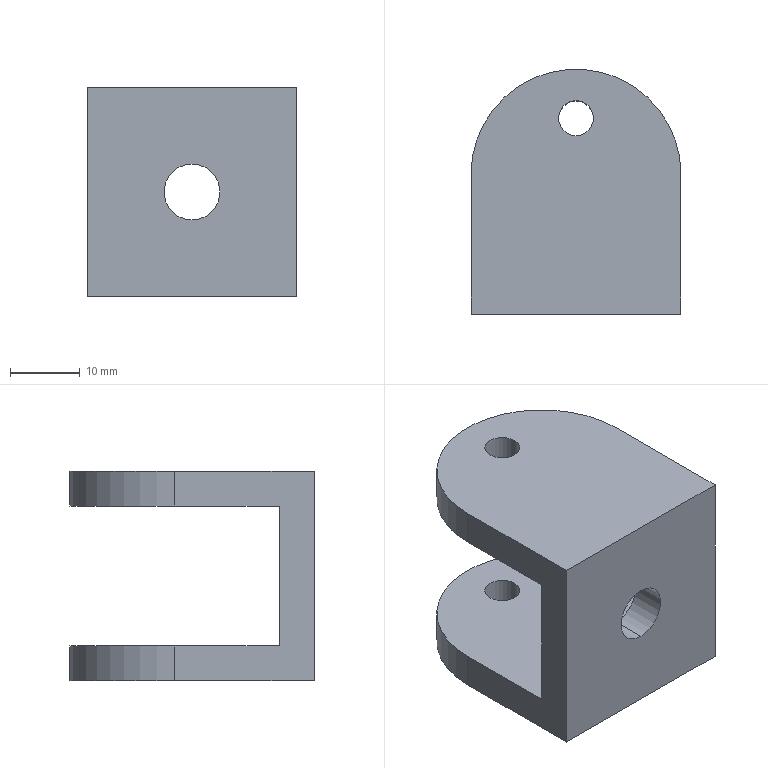Part | SolidWorks | features ICE 4, Extrusion 1 | 1 solid | 16 faces | box 30 x 35 x 30 mm | volume 12087 mm3 | cylinder 8 | plane 8 | commonest cylinder face diameters 5 x4 8 x2 30 x2
STEP:
#1=CARTESIAN_POINT('',(15.,5.,19.));
#2=VERTEX_POINT('',#1);
#3=CARTESIAN_POINT('',(15.,5.,11.));
#4=VERTEX_POINT('',#3);
#5=CARTESIAN_POINT('',(15.,5.,15.));
#6=DIRECTION('',(0.,-1.,0.));
#7=DIRECTION('',(1.,0.,0.));
#8=AXIS2_PLACEMENT_3D('',#5,#6,#7);
#9=CIRCLE('',#8,4.);
#10=EDGE_CURVE('',#2,#4,#9,.T.);
#11=ORIENTED_EDGE('',*,*,#10,.F.);
#12=CARTESIAN_POINT('',(15.,0.,19.));
#13=VERTEX_POINT('',#12);
#14=CARTESIAN_POINT('',(15.,40.,19.));
#15=DIRECTION('',(0.,-1.,0.));
#16=VECTOR('',#15,1000.);
#17=LINE('',#14,#16);
#18=EDGE_CURVE('',#2,#13,#17,.T.);
#19=ORIENTED_EDGE('',*,*,#18,.T.);
#20=CARTESIAN_POINT('',(15.,0.,11.));
#21=VERTEX_POINT('',#20);
#22=CARTESIAN_POINT('',(15.,0.,15.));
#23=DIRECTION('',(0.,-1.,0.));
#24=DIRECTION('',(0.,0.,-1.));
#25=AXIS2_PLACEMENT_3D('',#22,#23,#24);
#26=CIRCLE('',#25,4.);
#27=EDGE_CURVE('',#13,#21,#26,.T.);
#28=ORIENTED_EDGE('',*,*,#27,.T.);
#29=CARTESIAN_POINT('',(15.,40.,11.));
#30=DIRECTION('',(0.,-1.,0.));
#31=VECTOR('',#30,1000.);
#32=LINE('',#29,#31);
#33=EDGE_CURVE('',#4,#21,#32,.T.);
#34=ORIENTED_EDGE('',*,*,#33,.F.);
#35=EDGE_LOOP('',(#11,#19,#28,#34));
#36=FACE_OUTER_BOUND('',#35,.T.);
#37=CARTESIAN_POINT('',(15.,40.,15.));
#38=DIRECTION('',(0.,-1.,0.));
#39=DIRECTION('',(0.,0.,-1.));
#40=AXIS2_PLACEMENT_3D('',#37,#38,#39);
#41=CYLINDRICAL_SURFACE('',#40,4.);
#42=ADVANCED_FACE('',(#36),#41,.F.);
#43=CARTESIAN_POINT('',(17.5,28.,30.));
#44=VERTEX_POINT('',#43);
#45=CARTESIAN_POINT('',(12.5,28.,30.));
#46=VERTEX_POINT('',#45);
#47=CARTESIAN_POINT('',(15.,28.,30.));
#48=DIRECTION('',(0.,0.,-1.));
#49=DIRECTION('',(-1.,0.,0.));
#50=AXIS2_PLACEMENT_3D('',#47,#48,#49);
#51=CIRCLE('',#50,2.5);
#52=EDGE_CURVE('',#44,#46,#51,.T.);
#53=ORIENTED_EDGE('',*,*,#52,.F.);
#54=CARTESIAN_POINT('',(17.5,28.,25.));
#55=VERTEX_POINT('',#54);
#56=CARTESIAN_POINT('',(17.5,28.,40.));
#57=DIRECTION('',(0.,0.,-1.));
#58=VECTOR('',#57,1000.);
#59=LINE('',#56,#58);
#60=EDGE_CURVE('',#44,#55,#59,.T.);
#61=ORIENTED_EDGE('',*,*,#60,.T.);
#62=CARTESIAN_POINT('',(12.5,28.,25.));
#63=VERTEX_POINT('',#62);
#64=CARTESIAN_POINT('',(15.,28.,25.));
#65=DIRECTION('',(0.,0.,1.));
#66=DIRECTION('',(1.,0.,0.));
#67=AXIS2_PLACEMENT_3D('',#64,#65,#66);
#68=CIRCLE('',#67,2.5);
#69=EDGE_CURVE('',#63,#55,#68,.T.);
#70=ORIENTED_EDGE('',*,*,#69,.F.);
#71=CARTESIAN_POINT('',(12.5,28.,40.));
#72=DIRECTION('',(0.,0.,-1.));
#73=VECTOR('',#72,1000.);
#74=LINE('',#71,#73);
#75=EDGE_CURVE('',#46,#63,#74,.T.);
#76=ORIENTED_EDGE('',*,*,#75,.F.);
#77=EDGE_LOOP('',(#53,#61,#70,#76));
#78=FACE_OUTER_BOUND('',#77,.T.);
#79=CARTESIAN_POINT('',(15.,28.,40.));
#80=DIRECTION('',(0.,0.,-1.));
#81=DIRECTION('',(-1.,0.,0.));
#82=AXIS2_PLACEMENT_3D('',#79,#80,#81);
#83=CYLINDRICAL_SURFACE('',#82,2.5);
#84=ADVANCED_FACE('',(#78),#83,.F.);
#85=CARTESIAN_POINT('',(17.5,28.,5.));
#86=VERTEX_POINT('',#85);
#87=CARTESIAN_POINT('',(12.5,28.,5.));
#88=VERTEX_POINT('',#87);
#89=CARTESIAN_POINT('',(15.,28.,5.));
#90=DIRECTION('',(0.,0.,-1.));
#91=DIRECTION('',(0.,1.,0.));
#92=AXIS2_PLACEMENT_3D('',#89,#90,#91);
#93=CIRCLE('',#92,2.5);
#94=EDGE_CURVE('',#86,#88,#93,.T.);
#95=ORIENTED_EDGE('',*,*,#94,.F.);
#96=CARTESIAN_POINT('',(17.5,28.,0.));
#97=VERTEX_POINT('',#96);
#98=CARTESIAN_POINT('',(17.5,28.,40.));
#99=DIRECTION('',(0.,0.,-1.));
#100=VECTOR('',#99,1000.);
#101=LINE('',#98,#100);
#102=EDGE_CURVE('',#86,#97,#101,.T.);
#103=ORIENTED_EDGE('',*,*,#102,.T.);
#104=CARTESIAN_POINT('',(12.5,28.,0.));
#105=VERTEX_POINT('',#104);
#106=CARTESIAN_POINT('',(15.,28.,0.));
#107=DIRECTION('',(0.,0.,-1.));
#108=DIRECTION('',(-1.,0.,0.));
#109=AXIS2_PLACEMENT_3D('',#106,#107,#108);
#110=CIRCLE('',#109,2.5);
#111=EDGE_CURVE('',#97,#105,#110,.T.);
#112=ORIENTED_EDGE('',*,*,#111,.T.);
#113=CARTESIAN_POINT('',(12.5,28.,40.));
#114=DIRECTION('',(0.,0.,-1.));
#115=VECTOR('',#114,1000.);
#116=LINE('',#113,#115);
#117=EDGE_CURVE('',#88,#105,#116,.T.);
#118=ORIENTED_EDGE('',*,*,#117,.F.);
#119=EDGE_LOOP('',(#95,#103,#112,#118));
#120=FACE_OUTER_BOUND('',#119,.T.);
#121=CARTESIAN_POINT('',(15.,28.,40.));
#122=DIRECTION('',(0.,0.,-1.));
#123=DIRECTION('',(-1.,0.,0.));
#124=AXIS2_PLACEMENT_3D('',#121,#122,#123);
#125=CYLINDRICAL_SURFACE('',#124,2.5);
#126=ADVANCED_FACE('',(#120),#125,.F.);
#127=CARTESIAN_POINT('',(0.,20.,5.));
#128=VERTEX_POINT('',#127);
#129=CARTESIAN_POINT('',(0.,20.,0.));
#130=VERTEX_POINT('',#129);
#131=CARTESIAN_POINT('',(0.,20.,40.));
#132=DIRECTION('',(0.,0.,-1.));
#133=VECTOR('',#132,1000.);
#134=LINE('',#131,#133);
#135=EDGE_CURVE('',#128,#130,#134,.T.);
#136=ORIENTED_EDGE('',*,*,#135,.T.);
#137=CARTESIAN_POINT('',(0.,0.,0.));
#138=VERTEX_POINT('',#137);
#139=CARTESIAN_POINT('',(0.,0.,0.));
#140=DIRECTION('',(0.,-1.,0.));
#141=VECTOR('',#140,1000.);
#142=LINE('',#139,#141);
#143=EDGE_CURVE('',#130,#138,#142,.T.);
#144=ORIENTED_EDGE('',*,*,#143,.T.);
#145=CARTESIAN_POINT('',(0.,0.,30.));
#146=VERTEX_POINT('',#145);
#147=CARTESIAN_POINT('',(0.,0.,30.));
#148=DIRECTION('',(0.,0.,-1.));
#149=VECTOR('',#148,1000.);
#150=LINE('',#147,#149);
#151=EDGE_CURVE('',#146,#138,#150,.T.);
#152=ORIENTED_EDGE('',*,*,#151,.F.);
#153=CARTESIAN_POINT('',(0.,20.,30.));
#154=VERTEX_POINT('',#153);
#155=CARTESIAN_POINT('',(0.,0.,30.));
#156=DIRECTION('',(0.,-1.,0.));
#157=VECTOR('',#156,1000.);
#158=LINE('',#155,#157);
#159=EDGE_CURVE('',#154,#146,#158,.T.);
#160=ORIENTED_EDGE('',*,*,#159,.F.);
#161=CARTESIAN_POINT('',(0.,20.,25.));
#162=VERTEX_POINT('',#161);
#163=CARTESIAN_POINT('',(0.,20.,40.));
#164=DIRECTION('',(0.,0.,-1.));
#165=VECTOR('',#164,1000.);
#166=LINE('',#163,#165);
#167=EDGE_CURVE('',#154,#162,#166,.T.);
#168=ORIENTED_EDGE('',*,*,#167,.T.);
#169=CARTESIAN_POINT('',(0.,5.,25.));
#170=VERTEX_POINT('',#169);
#171=CARTESIAN_POINT('',(0.,0.,25.));
#172=DIRECTION('',(0.,-1.,0.));
#173=VECTOR('',#172,1000.);
#174=LINE('',#171,#173);
#175=EDGE_CURVE('',#162,#170,#174,.T.);
#176=ORIENTED_EDGE('',*,*,#175,.T.);
#177=CARTESIAN_POINT('',(0.,5.,5.));
#178=VERTEX_POINT('',#177);
#179=CARTESIAN_POINT('',(0.,5.,30.));
#180=DIRECTION('',(0.,0.,-1.));
#181=VECTOR('',#180,1000.);
#182=LINE('',#179,#181);
#183=EDGE_CURVE('',#170,#178,#182,.T.);
#184=ORIENTED_EDGE('',*,*,#183,.T.);
#185=CARTESIAN_POINT('',(0.,0.,5.));
#186=DIRECTION('',(0.,1.,0.));
#187=VECTOR('',#186,1000.);
#188=LINE('',#185,#187);
#189=EDGE_CURVE('',#178,#128,#188,.T.);
#190=ORIENTED_EDGE('',*,*,#189,.T.);
#191=EDGE_LOOP('',(#136,#144,#152,#160,#168,#176,#184,#190));
#192=FACE_OUTER_BOUND('',#191,.T.);
#193=CARTESIAN_POINT('',(0.,0.,30.));
#194=DIRECTION('',(1.,0.,0.));
#195=DIRECTION('',(0.,1.,0.));
#196=AXIS2_PLACEMENT_3D('',#193,#194,#195);
#197=PLANE('',#196);
#198=ADVANCED_FACE('',(#192),#197,.F.);
#199=CARTESIAN_POINT('',(15.,0.,15.));
#200=DIRECTION('',(0.,-1.,0.));
#201=DIRECTION('',(0.,0.,-1.));
#202=AXIS2_PLACEMENT_3D('',#199,#200,#201);
#203=CIRCLE('',#202,4.);
#204=EDGE_CURVE('',#21,#13,#203,.T.);
#205=ORIENTED_EDGE('',*,*,#204,.F.);
#206=ORIENTED_EDGE('',*,*,#27,.F.);
#207=EDGE_LOOP('',(#205,#206));
#208=FACE_BOUND('',#207,.T.);
#209=CARTESIAN_POINT('',(30.,0.,0.));
#210=VERTEX_POINT('',#209);
#211=CARTESIAN_POINT('',(0.,0.,0.));
#212=DIRECTION('',(1.,0.,0.));
#213=VECTOR('',#212,1000.);
#214=LINE('',#211,#213);
#215=EDGE_CURVE('',#138,#210,#214,.T.);
#216=ORIENTED_EDGE('',*,*,#215,.T.);
#217=CARTESIAN_POINT('',(30.,0.,30.));
#218=VERTEX_POINT('',#217);
#219=CARTESIAN_POINT('',(30.,0.,30.));
#220=DIRECTION('',(0.,0.,-1.));
#221=VECTOR('',#220,1000.);
#222=LINE('',#219,#221);
#223=EDGE_CURVE('',#218,#210,#222,.T.);
#224=ORIENTED_EDGE('',*,*,#223,.F.);
#225=CARTESIAN_POINT('',(0.,0.,30.));
#226=DIRECTION('',(1.,0.,0.));
#227=VECTOR('',#226,1000.);
#228=LINE('',#225,#227);
#229=EDGE_CURVE('',#146,#218,#228,.T.);
#230=ORIENTED_EDGE('',*,*,#229,.F.);
#231=ORIENTED_EDGE('',*,*,#151,.T.);
#232=EDGE_LOOP('',(#216,#224,#230,#231));
#233=FACE_OUTER_BOUND('',#232,.T.);
#234=CARTESIAN_POINT('',(0.,0.,30.));
#235=DIRECTION('',(0.,1.,0.));
#236=DIRECTION('',(0.,0.,1.));
#237=AXIS2_PLACEMENT_3D('',#234,#235,#236);
#238=PLANE('',#237);
#239=ADVANCED_FACE('',(#208,#233),#238,.F.);
#240=CARTESIAN_POINT('',(30.,20.,0.));
#241=VERTEX_POINT('',#240);
#242=CARTESIAN_POINT('',(30.,0.,0.));
#243=DIRECTION('',(0.,1.,0.));
#244=VECTOR('',#243,1000.);
#245=LINE('',#242,#244);
#246=EDGE_CURVE('',#210,#241,#245,.T.);
#247=ORIENTED_EDGE('',*,*,#246,.T.);
#248=CARTESIAN_POINT('',(30.,20.,5.));
#249=VERTEX_POINT('',#248);
#250=CARTESIAN_POINT('',(30.,20.,40.));
#251=DIRECTION('',(0.,0.,-1.));
#252=VECTOR('',#251,1000.);
#253=LINE('',#250,#252);
#254=EDGE_CURVE('',#249,#241,#253,.T.);
#255=ORIENTED_EDGE('',*,*,#254,.F.);
#256=CARTESIAN_POINT('',(30.,5.,5.));
#257=VERTEX_POINT('',#256);
#258=CARTESIAN_POINT('',(30.,40.,5.));
#259=DIRECTION('',(0.,1.,0.));
#260=VECTOR('',#259,1000.);
#261=LINE('',#258,#260);
#262=EDGE_CURVE('',#257,#249,#261,.T.);
#263=ORIENTED_EDGE('',*,*,#262,.F.);
#264=CARTESIAN_POINT('',(30.,5.,25.));
#265=VERTEX_POINT('',#264);
#266=CARTESIAN_POINT('',(30.,5.,25.));
#267=DIRECTION('',(0.,0.,-1.));
#268=VECTOR('',#267,1000.);
#269=LINE('',#266,#268);
#270=EDGE_CURVE('',#265,#257,#269,.T.);
#271=ORIENTED_EDGE('',*,*,#270,.F.);
#272=CARTESIAN_POINT('',(30.,20.,25.));
#273=VERTEX_POINT('',#272);
#274=CARTESIAN_POINT('',(30.,40.,25.));
#275=DIRECTION('',(0.,-1.,0.));
#276=VECTOR('',#275,1000.);
#277=LINE('',#274,#276);
#278=EDGE_CURVE('',#273,#265,#277,.T.);
#279=ORIENTED_EDGE('',*,*,#278,.F.);
#280=CARTESIAN_POINT('',(30.,20.,30.));
#281=VERTEX_POINT('',#280);
#282=CARTESIAN_POINT('',(30.,20.,40.));
#283=DIRECTION('',(0.,0.,-1.));
#284=VECTOR('',#283,1000.);
#285=LINE('',#282,#284);
#286=EDGE_CURVE('',#281,#273,#285,.T.);
#287=ORIENTED_EDGE('',*,*,#286,.F.);
#288=CARTESIAN_POINT('',(30.,0.,30.));
#289=DIRECTION('',(0.,1.,0.));
#290=VECTOR('',#289,1000.);
#291=LINE('',#288,#290);
#292=EDGE_CURVE('',#218,#281,#291,.T.);
#293=ORIENTED_EDGE('',*,*,#292,.F.);
#294=ORIENTED_EDGE('',*,*,#223,.T.);
#295=EDGE_LOOP('',(#247,#255,#263,#271,#279,#287,#293,#294));
#296=FACE_OUTER_BOUND('',#295,.T.);
#297=CARTESIAN_POINT('',(30.,0.,30.));
#298=DIRECTION('',(-1.,0.,0.));
#299=DIRECTION('',(0.,-1.,0.));
#300=AXIS2_PLACEMENT_3D('',#297,#298,#299);
#301=PLANE('',#300);
#302=ADVANCED_FACE('',(#296),#301,.F.);
#303=CARTESIAN_POINT('',(15.,28.,30.));
#304=DIRECTION('',(0.,0.,-1.));
#305=DIRECTION('',(-1.,0.,0.));
#306=AXIS2_PLACEMENT_3D('',#303,#304,#305);
#307=CIRCLE('',#306,2.5);
#308=EDGE_CURVE('',#46,#44,#307,.T.);
#309=ORIENTED_EDGE('',*,*,#308,.T.);
#310=ORIENTED_EDGE('',*,*,#52,.T.);
#311=EDGE_LOOP('',(#309,#310));
#312=FACE_BOUND('',#311,.T.);
#313=ORIENTED_EDGE('',*,*,#292,.T.);
#314=CARTESIAN_POINT('',(15.,20.,30.));
#315=DIRECTION('',(0.,0.,1.));
#316=DIRECTION('',(-1.,0.,0.));
#317=AXIS2_PLACEMENT_3D('',#314,#315,#316);
#318=CIRCLE('',#317,15.);
#319=EDGE_CURVE('',#281,#154,#318,.T.);
#320=ORIENTED_EDGE('',*,*,#319,.T.);
#321=ORIENTED_EDGE('',*,*,#159,.T.);
#322=ORIENTED_EDGE('',*,*,#229,.T.);
#323=EDGE_LOOP('',(#313,#320,#321,#322));
#324=FACE_OUTER_BOUND('',#323,.T.);
#325=CARTESIAN_POINT('',(0.,40.,30.));
#326=DIRECTION('',(0.,0.,-1.));
#327=DIRECTION('',(-1.,0.,0.));
#328=AXIS2_PLACEMENT_3D('',#325,#326,#327);
#329=PLANE('',#328);
#330=ADVANCED_FACE('',(#312,#324),#329,.F.);
#331=CARTESIAN_POINT('',(15.,28.,0.));
#332=DIRECTION('',(0.,0.,-1.));
#333=DIRECTION('',(-1.,0.,0.));
#334=AXIS2_PLACEMENT_3D('',#331,#332,#333);
#335=CIRCLE('',#334,2.5);
#336=EDGE_CURVE('',#105,#97,#335,.T.);
#337=ORIENTED_EDGE('',*,*,#336,.F.);
#338=ORIENTED_EDGE('',*,*,#111,.F.);
#339=EDGE_LOOP('',(#337,#338));
#340=FACE_BOUND('',#339,.T.);
#341=CARTESIAN_POINT('',(15.,20.,0.));
#342=DIRECTION('',(0.,0.,1.));
#343=DIRECTION('',(-1.,0.,0.));
#344=AXIS2_PLACEMENT_3D('',#341,#342,#343);
#345=CIRCLE('',#344,15.);
#346=EDGE_CURVE('',#241,#130,#345,.T.);
#347=ORIENTED_EDGE('',*,*,#346,.F.);
#348=ORIENTED_EDGE('',*,*,#246,.F.);
#349=ORIENTED_EDGE('',*,*,#215,.F.);
#350=ORIENTED_EDGE('',*,*,#143,.F.);
#351=EDGE_LOOP('',(#347,#348,#349,#350));
#352=FACE_OUTER_BOUND('',#351,.T.);
#353=CARTESIAN_POINT('',(0.,40.,0.));
#354=DIRECTION('',(0.,0.,-1.));
#355=DIRECTION('',(-1.,0.,0.));
#356=AXIS2_PLACEMENT_3D('',#353,#354,#355);
#357=PLANE('',#356);
#358=ADVANCED_FACE('',(#340,#352),#357,.T.);
#359=CARTESIAN_POINT('',(15.,5.,15.));
#360=DIRECTION('',(0.,-1.,0.));
#361=DIRECTION('',(1.,0.,0.));
#362=AXIS2_PLACEMENT_3D('',#359,#360,#361);
#363=CIRCLE('',#362,4.);
#364=EDGE_CURVE('',#4,#2,#363,.T.);
#365=ORIENTED_EDGE('',*,*,#364,.T.);
#366=ORIENTED_EDGE('',*,*,#10,.T.);
#367=EDGE_LOOP('',(#365,#366));
#368=FACE_BOUND('',#367,.T.);
#369=CARTESIAN_POINT('',(-10.,5.,25.));
#370=DIRECTION('',(1.,0.,0.));
#371=VECTOR('',#370,1000.);
#372=LINE('',#369,#371);
#373=EDGE_CURVE('',#170,#265,#372,.T.);
#374=ORIENTED_EDGE('',*,*,#373,.T.);
#375=ORIENTED_EDGE('',*,*,#270,.T.);
#376=CARTESIAN_POINT('',(-10.,5.,5.));
#377=DIRECTION('',(1.,0.,0.));
#378=VECTOR('',#377,1000.);
#379=LINE('',#376,#378);
#380=EDGE_CURVE('',#178,#257,#379,.T.);
#381=ORIENTED_EDGE('',*,*,#380,.F.);
#382=ORIENTED_EDGE('',*,*,#183,.F.);
#383=EDGE_LOOP('',(#374,#375,#381,#382));
#384=FACE_OUTER_BOUND('',#383,.T.);
#385=CARTESIAN_POINT('',(-10.,5.,25.));
#386=DIRECTION('',(0.,-1.,0.));
#387=DIRECTION('',(1.,0.,0.));
#388=AXIS2_PLACEMENT_3D('',#385,#386,#387);
#389=PLANE('',#388);
#390=ADVANCED_FACE('',(#368,#384),#389,.F.);
#391=ORIENTED_EDGE('',*,*,#69,.T.);
#392=CARTESIAN_POINT('',(15.,28.,25.));
#393=DIRECTION('',(0.,0.,1.));
#394=DIRECTION('',(1.,0.,0.));
#395=AXIS2_PLACEMENT_3D('',#392,#393,#394);
#396=CIRCLE('',#395,2.5);
#397=EDGE_CURVE('',#55,#63,#396,.T.);
#398=ORIENTED_EDGE('',*,*,#397,.T.);
#399=EDGE_LOOP('',(#391,#398));
#400=FACE_BOUND('',#399,.T.);
#401=ORIENTED_EDGE('',*,*,#175,.F.);
#402=CARTESIAN_POINT('',(15.,20.,25.));
#403=DIRECTION('',(0.,0.,-1.));
#404=DIRECTION('',(1.,0.,0.));
#405=AXIS2_PLACEMENT_3D('',#402,#403,#404);
#406=CIRCLE('',#405,15.);
#407=EDGE_CURVE('',#162,#273,#406,.T.);
#408=ORIENTED_EDGE('',*,*,#407,.T.);
#409=ORIENTED_EDGE('',*,*,#278,.T.);
#410=ORIENTED_EDGE('',*,*,#373,.F.);
#411=EDGE_LOOP('',(#401,#408,#409,#410));
#412=FACE_OUTER_BOUND('',#411,.T.);
#413=CARTESIAN_POINT('',(-10.,40.,25.));
#414=DIRECTION('',(0.,0.,1.));
#415=DIRECTION('',(1.,0.,0.));
#416=AXIS2_PLACEMENT_3D('',#413,#414,#415);
#417=PLANE('',#416);
#418=ADVANCED_FACE('',(#400,#412),#417,.F.);
#419=CARTESIAN_POINT('',(15.,28.,5.));
#420=DIRECTION('',(0.,0.,-1.));
#421=DIRECTION('',(0.,1.,0.));
#422=AXIS2_PLACEMENT_3D('',#419,#420,#421);
#423=CIRCLE('',#422,2.5);
#424=EDGE_CURVE('',#88,#86,#423,.T.);
#425=ORIENTED_EDGE('',*,*,#424,.T.);
#426=ORIENTED_EDGE('',*,*,#94,.T.);
#427=EDGE_LOOP('',(#425,#426));
#428=FACE_BOUND('',#427,.T.);
#429=ORIENTED_EDGE('',*,*,#262,.T.);
#430=CARTESIAN_POINT('',(15.,20.,5.));
#431=DIRECTION('',(0.,0.,1.));
#432=DIRECTION('',(0.,1.,0.));
#433=AXIS2_PLACEMENT_3D('',#430,#431,#432);
#434=CIRCLE('',#433,15.);
#435=EDGE_CURVE('',#249,#128,#434,.T.);
#436=ORIENTED_EDGE('',*,*,#435,.T.);
#437=ORIENTED_EDGE('',*,*,#189,.F.);
#438=ORIENTED_EDGE('',*,*,#380,.T.);
#439=EDGE_LOOP('',(#429,#436,#437,#438));
#440=FACE_OUTER_BOUND('',#439,.T.);
#441=CARTESIAN_POINT('',(-10.,40.,5.));
#442=DIRECTION('',(0.,0.,-1.));
#443=DIRECTION('',(0.,1.,0.));
#444=AXIS2_PLACEMENT_3D('',#441,#442,#443);
#445=PLANE('',#444);
#446=ADVANCED_FACE('',(#428,#440),#445,.F.);
#447=ORIENTED_EDGE('',*,*,#254,.T.);
#448=ORIENTED_EDGE('',*,*,#346,.T.);
#449=ORIENTED_EDGE('',*,*,#135,.F.);
#450=ORIENTED_EDGE('',*,*,#435,.F.);
#451=EDGE_LOOP('',(#447,#448,#449,#450));
#452=FACE_OUTER_BOUND('',#451,.T.);
#453=CARTESIAN_POINT('',(15.,20.,40.));
#454=DIRECTION('',(0.,0.,-1.));
#455=DIRECTION('',(-1.,0.,0.));
#456=AXIS2_PLACEMENT_3D('',#453,#454,#455);
#457=CYLINDRICAL_SURFACE('',#456,15.);
#458=ADVANCED_FACE('',(#452),#457,.T.);
#459=ORIENTED_EDGE('',*,*,#286,.T.);
#460=ORIENTED_EDGE('',*,*,#407,.F.);
#461=ORIENTED_EDGE('',*,*,#167,.F.);
#462=ORIENTED_EDGE('',*,*,#319,.F.);
#463=EDGE_LOOP('',(#459,#460,#461,#462));
#464=FACE_OUTER_BOUND('',#463,.T.);
#465=CARTESIAN_POINT('',(15.,20.,40.));
#466=DIRECTION('',(0.,0.,-1.));
#467=DIRECTION('',(-1.,0.,0.));
#468=AXIS2_PLACEMENT_3D('',#465,#466,#467);
#469=CYLINDRICAL_SURFACE('',#468,15.);
#470=ADVANCED_FACE('',(#464),#469,.T.);
#471=ORIENTED_EDGE('',*,*,#102,.F.);
#472=ORIENTED_EDGE('',*,*,#424,.F.);
#473=ORIENTED_EDGE('',*,*,#117,.T.);
#474=ORIENTED_EDGE('',*,*,#336,.T.);
#475=EDGE_LOOP('',(#471,#472,#473,#474));
#476=FACE_OUTER_BOUND('',#475,.T.);
#477=CARTESIAN_POINT('',(15.,28.,40.));
#478=DIRECTION('',(0.,0.,-1.));
#479=DIRECTION('',(-1.,0.,0.));
#480=AXIS2_PLACEMENT_3D('',#477,#478,#479);
#481=CYLINDRICAL_SURFACE('',#480,2.5);
#482=ADVANCED_FACE('',(#476),#481,.F.);
#483=ORIENTED_EDGE('',*,*,#60,.F.);
#484=ORIENTED_EDGE('',*,*,#308,.F.);
#485=ORIENTED_EDGE('',*,*,#75,.T.);
#486=ORIENTED_EDGE('',*,*,#397,.F.);
#487=EDGE_LOOP('',(#483,#484,#485,#486));
#488=FACE_OUTER_BOUND('',#487,.T.);
#489=CARTESIAN_POINT('',(15.,28.,40.));
#490=DIRECTION('',(0.,0.,-1.));
#491=DIRECTION('',(-1.,0.,0.));
#492=AXIS2_PLACEMENT_3D('',#489,#490,#491);
#493=CYLINDRICAL_SURFACE('',#492,2.5);
#494=ADVANCED_FACE('',(#488),#493,.F.);
#495=ORIENTED_EDGE('',*,*,#18,.F.);
#496=ORIENTED_EDGE('',*,*,#364,.F.);
#497=ORIENTED_EDGE('',*,*,#33,.T.);
#498=ORIENTED_EDGE('',*,*,#204,.T.);
#499=EDGE_LOOP('',(#495,#496,#497,#498));
#500=FACE_OUTER_BOUND('',#499,.T.);
#501=CARTESIAN_POINT('',(15.,40.,15.));
#502=DIRECTION('',(0.,-1.,0.));
#503=DIRECTION('',(0.,0.,-1.));
#504=AXIS2_PLACEMENT_3D('',#501,#502,#503);
#505=CYLINDRICAL_SURFACE('',#504,4.);
#506=ADVANCED_FACE('',(#500),#505,.F.);
#507=CLOSED_SHELL('',(#42,#84,#126,#198,#239,#302,#330,#358,#390,#418,#446,#458,#470,#482,#494,#506));
#508=MANIFOLD_SOLID_BREP('',#507);
#509=CARTESIAN_POINT('',(0.,0.,0.));
#510=DIRECTION('',(0.,0.,1.));
#511=DIRECTION('',(1.,0.,0.));
#512=AXIS2_PLACEMENT_3D('',#509,#510,#511);
#513=(LENGTH_UNIT()NAMED_UNIT(*)SI_UNIT(.MILLI.,.METRE.));
#514=UNCERTAINTY_MEASURE_WITH_UNIT(LENGTH_MEASURE(0.00001),#513,'','');
#515=(NAMED_UNIT(*)PLANE_ANGLE_UNIT()SI_UNIT($,.RADIAN.));
#516=(NAMED_UNIT(*)SI_UNIT($,.STERADIAN.)SOLID_ANGLE_UNIT());
#517=(GEOMETRIC_REPRESENTATION_CONTEXT(3)GLOBAL_UNCERTAINTY_ASSIGNED_CONTEXT((#514))GLOBAL_UNIT_ASSIGNED_CONTEXT((#513,#515,#516))REPRESENTATION_CONTEXT('',''));
#518=ADVANCED_BREP_SHAPE_REPRESENTATION('',(#508,#512),#517);